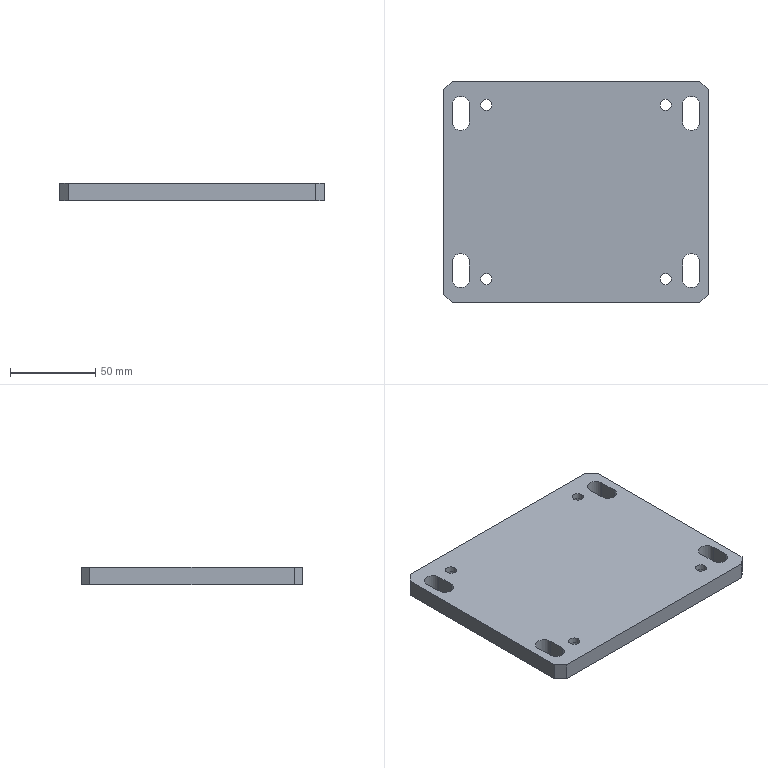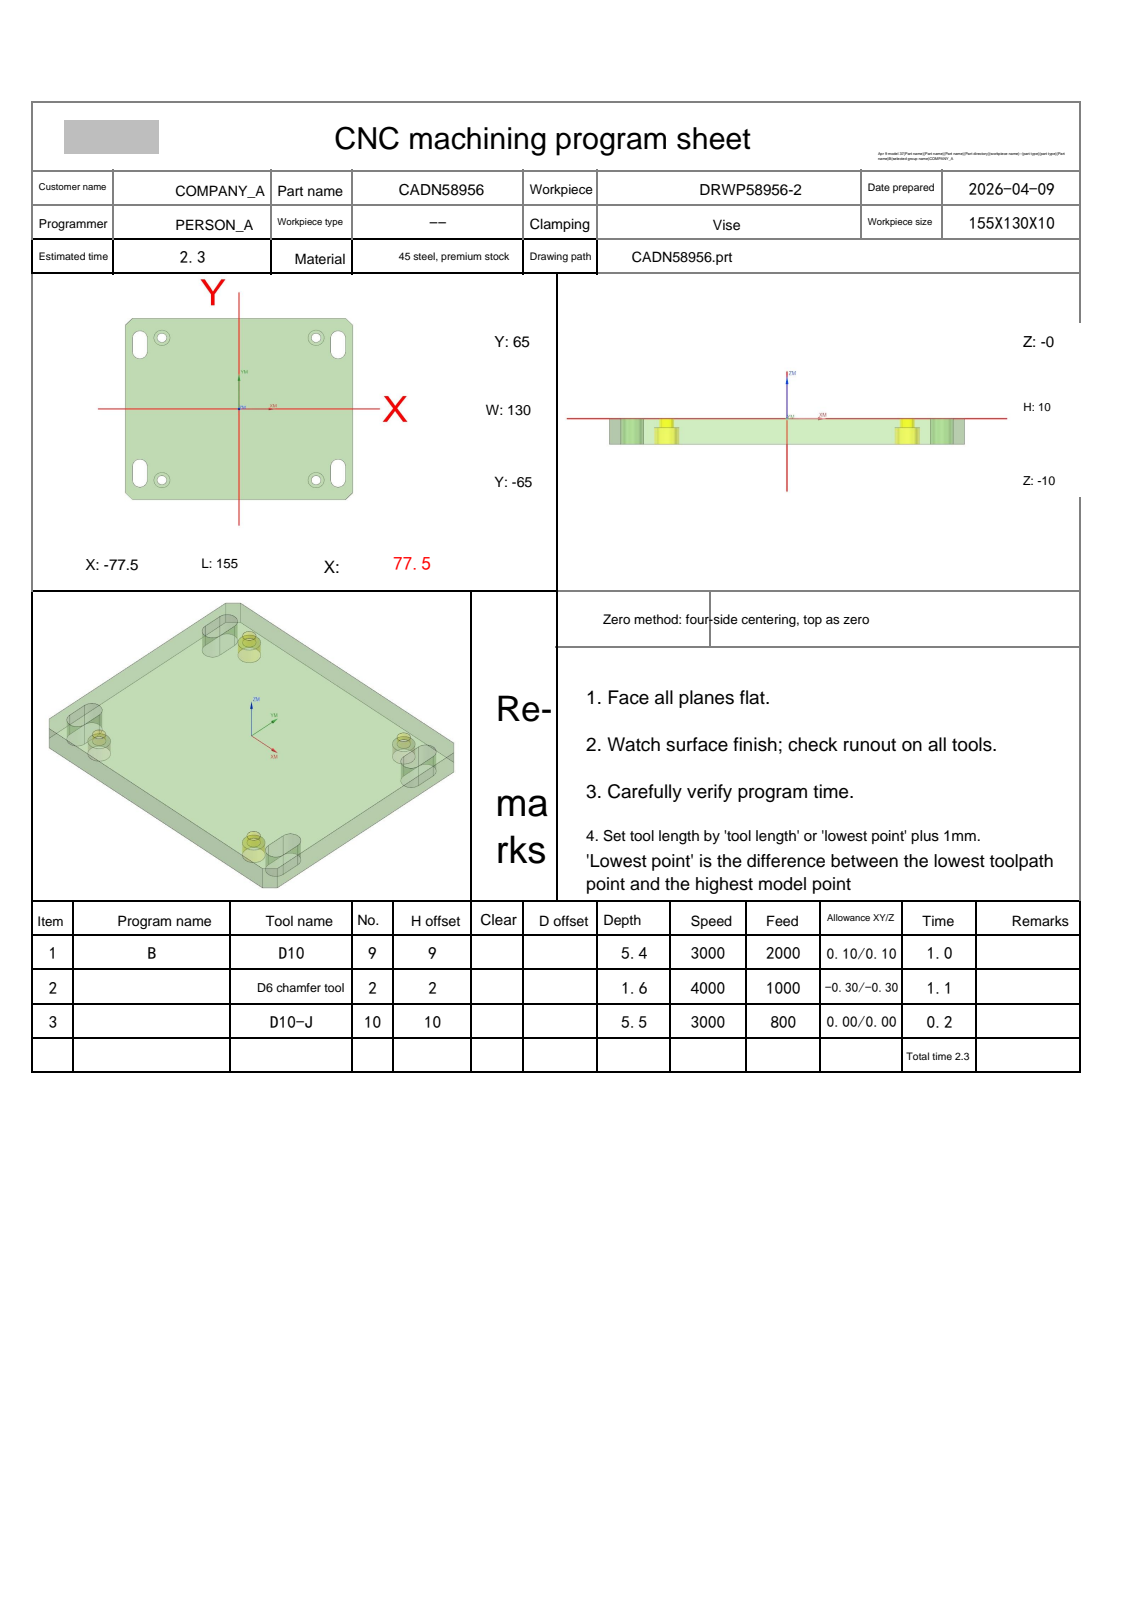NC program | NX | posted by the shop | part box 155 x 130 x 10 mm
Whole program:
%
O0001
(Machine time: 2.75 MIN)
(===Total Tool:3===)
(T9=D10     D=10.  R=0.   D-  H09 Z=-5.4  )
(T2=D6 chamfer tool   D=6.   R=0.   D-  H02 Z=-1.6  )
(T10=D10-J  D=10.  R=0.   D-  H10 Z=-5.5  )
G80 G90 G17 G49 G40
G91 G28 Z0
M01
N1 T09 M06
(D10  D=10. R=0. H=09 ce=0.10 di=0.10)
G00 G90 G54 X69.742 Y74.97 M03 S3000
G43 H09 Z20.
M08
Z-.3
G01 X76.106 Y68.606 F2000.
X81.106 Y63.606
X87.47 Y57.242
G00 Z-.6
G01 X81.106 Y63.606
X76.106 Y68.606
X69.742 Y74.97
G00 Z-.9
G01 X76.106 Y68.606
X81.106 Y63.606
X87.47 Y57.242
G00 Z-1.2
G01 X81.106 Y63.606
X76.106 Y68.606
X69.742 Y74.97
G00 Z-1.5
G01 X76.106 Y68.606
X81.106 Y63.606
X87.47 Y57.242
G00 Z-1.8
G01 X81.106 Y63.606
X76.106 Y68.606
X69.742 Y74.97
G00 Z-2.1
G01 X76.106 Y68.606
X81.106 Y63.606
X87.47 Y57.242
G00 Z-2.4
G01 X81.106 Y63.606
X76.106 Y68.606
X69.742 Y74.97
G00 Z-2.7
G01 X76.106 Y68.606
X81.106 Y63.606
X87.47 Y57.242
G00 Z-3.
G01 X81.106 Y63.606
X76.106 Y68.606
X69.742 Y74.97
G00 Z-3.3
G01 X76.106 Y68.606
X81.106 Y63.606
X87.47 Y57.242
G00 Z-3.6
G01 X81.106 Y63.606
X76.106 Y68.606
X69.742 Y74.97
G00 Z-3.9
G01 X76.106 Y68.606
X81.106 Y63.606
X87.47 Y57.242
G00 Z-4.2
G01 X81.106 Y63.606
X76.106 Y68.606
X69.742 Y74.97
G00 Z-4.5
G01 X76.106 Y68.606
X81.106 Y63.606
X87.47 Y57.242
G00 Z-4.8
G01 X81.106 Y63.606
X76.106 Y68.606
X69.742 Y74.97
G00 Z-5.1
G01 X76.106 Y68.606
X81.106 Y63.606
X87.47 Y57.242
G00 Z-5.4
G01 X81.106 Y63.606
X76.106 Y68.606
X69.742 Y74.97
G00 Z20.
X87.47 Y-57.242
Z-.3
G01 X81.106 Y-63.606
X76.106 Y-68.606
X69.742 Y-74.97
G00 Z-.6
G01 X76.106 Y-68.606
X81.106 Y-63.606
X87.47 Y-57.242
G00 Z-.9
G01 X81.106 Y-63.606
X76.106 Y-68.606
X69.742 Y-74.97
G00 Z-1.2
G01 X76.106 Y-68.606
X81.106 Y-63.606
X87.47 Y-57.242
G00 Z-1.5
G01 X81.106 Y-63.606
X76.106 Y-68.606
X69.742 Y-74.97
G00 Z-1.8
G01 X76.106 Y-68.606
X81.106 Y-63.606
X87.47 Y-57.242
G00 Z-2.1
G01 X81.106 Y-63.606
X76.106 Y-68.606
X69.742 Y-74.97
G00 Z-2.4
G01 X76.106 Y-68.606
X81.106 Y-63.606
X87.47 Y-57.242
G00 Z-2.7
G01 X81.106 Y-63.606
X76.106 Y-68.606
X69.742 Y-74.97
G00 Z-3.
G01 X76.106 Y-68.606
X81.106 Y-63.606
X87.47 Y-57.242
G00 Z-3.3
G01 X81.106 Y-63.606
X76.106 Y-68.606
X69.742 Y-74.97
G00 Z-3.6
G01 X76.106 Y-68.606
X81.106 Y-63.606
X87.47 Y-57.242
G00 Z-3.9
G01 X81.106 Y-63.606
X76.106 Y-68.606
X69.742 Y-74.97
G00 Z-4.2
G01 X76.106 Y-68.606
X81.106 Y-63.606
X87.47 Y-57.242
G00 Z-4.5
G01 X81.106 Y-63.606
X76.106 Y-68.606
X69.742 Y-74.97
G00 Z-4.8
G01 X76.106 Y-68.606
X81.106 Y-63.606
X87.47 Y-57.242
G00 Z-5.1
G01 X81.106 Y-63.606
X76.106 Y-68.606
X69.742 Y-74.97
G00 Z-5.4
G01 X76.106 Y-68.606
X81.106 Y-63.606
X87.47 Y-57.242
G00 Z20.
X-69.742 Y-74.97
Z-.3
G01 X-76.106 Y-68.606
X-81.106 Y-63.606
X-87.47 Y-57.242
G00 Z-.6
G01 X-81.106 Y-63.606
X-76.106 Y-68.606
X-69.742 Y-74.97
G00 Z-.9
G01 X-76.106 Y-68.606
X-81.106 Y-63.606
X-87.47 Y-57.242
G00 Z-1.2
G01 X-81.106 Y-63.606
X-76.106 Y-68.606
X-69.742 Y-74.97
G00 Z-1.5
G01 X-76.106 Y-68.606
X-81.106 Y-63.606
X-87.47 Y-57.242
G00 Z-1.8
G01 X-81.106 Y-63.606
X-76.106 Y-68.606
X-69.742 Y-74.97
G00 Z-2.1
G01 X-76.106 Y-68.606
X-81.106 Y-63.606
X-87.47 Y-57.242
G00 Z-2.4
G01 X-81.106 Y-63.606
X-76.106 Y-68.606
X-69.742 Y-74.97
G00 Z-2.7
G01 X-76.106 Y-68.606
X-81.106 Y-63.606
X-87.47 Y-57.242
G00 Z-3.
G01 X-81.106 Y-63.606
X-76.106 Y-68.606
X-69.742 Y-74.97
G00 Z-3.3
G01 X-76.106 Y-68.606
X-81.106 Y-63.606
X-87.47 Y-57.242
G00 Z-3.6
G01 X-81.106 Y-63.606
X-76.106 Y-68.606
X-69.742 Y-74.97
G00 Z-3.9
G01 X-76.106 Y-68.606
X-81.106 Y-63.606
X-87.47 Y-57.242
G00 Z-4.2
G01 X-81.106 Y-63.606
X-76.106 Y-68.606
X-69.742 Y-74.97
G00 Z-4.5
G01 X-76.106 Y-68.606
X-81.106 Y-63.606
X-87.47 Y-57.242
G00 Z-4.8
G01 X-81.106 Y-63.606
X-76.106 Y-68.606
X-69.742 Y-74.97
G00 Z-5.1
G01 X-76.106 Y-68.606
X-81.106 Y-63.606
X-87.47 Y-57.242
G00 Z-5.4
G01 X-81.106 Y-63.606
X-76.106 Y-68.606
X-69.742 Y-74.97
G00 Z20.
X-87.47 Y57.242
Z-.3
G01 X-81.106 Y63.606
X-76.106 Y68.606
X-69.742 Y74.97
G00 Z-.6
G01 X-76.106 Y68.606
X-81.106 Y63.606
X-87.47 Y57.242
G00 Z-.9
G01 X-81.106 Y63.606
X-76.106 Y68.606
X-69.742 Y74.97
G00 Z-1.2
G01 X-76.106 Y68.606
X-81.106 Y63.606
X-87.47 Y57.242
G00 Z-1.5
G01 X-81.106 Y63.606
X-76.106 Y68.606
X-69.742 Y74.97
G00 Z-1.8
G01 X-76.106 Y68.606
X-81.106 Y63.606
X-87.47 Y57.242
G00 Z-2.1
G01 X-81.106 Y63.606
X-76.106 Y68.606
X-69.742 Y74.97
G00 Z-2.4
G01 X-76.106 Y68.606
X-81.106 Y63.606
X-87.47 Y57.242
G00 Z-2.7
G01 X-81.106 Y63.606
X-76.106 Y68.606
X-69.742 Y74.97
G00 Z-3.
G01 X-76.106 Y68.606
X-81.106 Y63.606
X-87.47 Y57.242
G00 Z-3.3
G01 X-81.106 Y63.606
X-76.106 Y68.606
X-69.742 Y74.97
G00 Z-3.6
G01 X-76.106 Y68.606
X-81.106 Y63.606
X-87.47 Y57.242
G00 Z-3.9
G01 X-81.106 Y63.606
X-76.106 Y68.606
X-69.742 Y74.97
G00 Z-4.2
G01 X-76.106 Y68.606
X-81.106 Y63.606
X-87.47 Y57.242
G00 Z-4.5
G01 X-81.106 Y63.606
X-76.106 Y68.606
X-69.742 Y74.97
G00 Z-4.8
G01 X-76.106 Y68.606
X-81.106 Y63.606
X-87.47 Y57.242
G00 Z-5.1
G01 X-81.106 Y63.606
X-76.106 Y68.606
X-69.742 Y74.97
G00 Z-5.4
G01 X-76.106 Y68.606
X-81.106 Y63.606
X-87.47 Y57.242
G00 Z20.
G91 G28 Z0.0
M05
M09
G91 G28 Z0.0
M01
N2 T02 M06
(D6 chamfer tool  D=6. R=0. H=02 ce=-0.30 di=-0.80)
G00 G90 G54 X-52.227 Y50.09 M03 S4000
G43 H02 Z20.
M08
Z-1.1
G01 Z-1.6 F600.
X-52.05 Y49.5
G03 X-50.55 Y51. I0.0 J1.5
X-52.5 Y52.95 I-1.95 J0.0
X-54.45 Y51. I0.0 J-1.95
X-52.5 Y49.05 I1.95 J0.0
X-50.55 Y51. I0.0 J1.95
X-52.05 Y52.5 I-1.5 J0.0
G01 X-52.227 Y51.91
Z-1.1
G00 Z20.
Y-51.91
Z-1.1
G01 Z-1.6
X-52.05 Y-52.5
G03 X-50.55 Y-51. I0.0 J1.5
X-52.5 Y-49.05 I-1.95 J0.0
X-54.45 Y-51. I0.0 J-1.95
X-52.5 Y-52.95 I1.95 J0.0
X-50.55 Y-51. I0.0 J1.95
X-52.05 Y-49.5 I-1.5 J0.0
G01 X-52.227 Y-50.09
Z-1.1
G00 Z20.
X52.773 Y-51.91
Z-1.1
G01 Z-1.6
X52.95 Y-52.5
G03 X54.45 Y-51. I0.0 J1.5
X52.5 Y-49.05 I-1.95 J0.0
X50.55 Y-51. I0.0 J-1.95
X52.5 Y-52.95 I1.95 J0.0
X54.45 Y-51. I0.0 J1.95
X52.95 Y-49.5 I-1.5 J0.0
G01 X52.773 Y-50.09
Z-1.1
G00 Z20.
Y50.09
Z-1.1
G01 Z-1.6
X52.95 Y49.5
G03 X54.45 Y51. I0.0 J1.5
X52.5 Y52.95 I-1.95 J0.0
X50.55 Y51. I0.0 J-1.95
X52.5 Y49.05 I1.95 J0.0
X54.45 Y51. I0.0 J1.95
X52.95 Y52.5 I-1.5 J0.0
G01 X52.773 Y51.91
Z-1.1
G00 Z20.
G00 G90 X.386 Y-66.227 M03 S3500
Z20.
Z.172
G01 Z-1.199 F1000.
G03 X.1 Y-66.027 I-1.286 J-1.532
G01 X.054 Y-65.997
X0.0 Y-66.
X-72.5
X-72.759 Y-65.966
X-73. Y-65.866
X-73.207 Y-65.707
X-78.207 Y-60.707
X-78.366 Y-60.5
X-78.466 Y-60.259
X-78.5 Y-60.
Y60.
X-78.466 Y60.259
X-78.366 Y60.5
X-78.207 Y60.707
X-73.207 Y65.707
X-73. Y65.866
X-72.759 Y65.966
X-72.5 Y66.
X72.5
X72.759 Y65.966
X73. Y65.866
X73.207 Y65.707
X78.207 Y60.707
X78.366 Y60.5
X78.466 Y60.259
X78.5 Y60.
Y-60.
X78.466 Y-60.259
X78.366 Y-60.5
X78.207 Y-60.707
X73.207 Y-65.707
X73. Y-65.866
X72.759 Y-65.966
X72.5 Y-66.
X0.0
X-.054 Y-65.997
X-.1 Y-66.027
G03 X-.386 Y-66.227 I1. J-1.732
G01 Z.172
G00 Z10.
X-50.442 Y-51.404
Z.249
G01 Z-1.199
G03 X-50.268 Y-51.102 I-1.638 J1.147
G01 X-50.242 Y-51.054
X-50.25 Y-51.
G03 X-52.5 Y-48.75 I-2.25 J0.0
X-54.75 Y-51. I0.0 J-2.25
X-52.5 Y-53.25 I2.25 J0.0
X-50.25 Y-51. I0.0 J2.25
G01 X-50.242 Y-50.946
X-50.268 Y-50.898
G03 X-50.442 Y-50.596 I-1.813 J-.845
G01 Z.255
G00 Z10.
X-63.727 Y-46.386
Z.172
G01 Z-1.199
G03 X-63.527 Y-46.1 I-1.532 J1.286
G01 X-63.497 Y-46.054
X-63.5 Y-46.
Y-41.
G03 X-67.5 Y-37. I-4. J0.0
X-71.5 Y-41. I0.0 J-4.
G01 Y-51.
G03 X-67.5 Y-55. I4. J0.0
X-63.5 Y-51. I0.0 J4.
G01 Y-46.
X-63.497 Y-45.946
X-63.527 Y-45.9
G03 X-63.727 Y-45.614 I-1.732 J-1.
G01 Z.172
G00 Z10.
Y45.614
Z.172
G01 Z-1.199
G03 X-63.527 Y45.9 I-1.532 J1.286
G01 X-63.497 Y45.946
X-63.5 Y46.
Y51.
G03 X-67.5 Y55. I-4. J0.0
X-71.5 Y51. I0.0 J-4.
G01 Y41.
G03 X-67.5 Y37. I4. J0.0
X-63.5 Y41. I0.0 J4.
G01 Y46.
X-63.497 Y46.054
X-63.527 Y46.1
G03 X-63.727 Y46.386 I-1.732 J-1.
G01 Z.172
G00 Z10.
X-50.442 Y50.596
Z.249
G01 Z-1.199
G03 X-50.268 Y50.898 I-1.638 J1.147
G01 X-50.242 Y50.946
X-50.25 Y51.
G03 X-52.5 Y53.25 I-2.25 J0.0
X-54.75 Y51. I0.0 J-2.25
X-52.5 Y48.75 I2.25 J0.0
X-50.25 Y51. I0.0 J2.25
G01 X-50.242 Y51.054
X-50.268 Y51.102
G03 X-50.442 Y51.404 I-1.813 J-.845
G01 Z.255
G00 Z10.
X54.558 Y50.596
Z.255
G01 Z-1.199
G03 X54.732 Y50.898 I-1.638 J1.147
G01 X54.758 Y50.946
X54.75 Y51.
G03 X52.5 Y53.25 I-2.25 J0.0
X50.25 Y51. I0.0 J-2.25
X52.5 Y48.75 I2.25 J0.0
X54.75 Y51. I0.0 J2.25
G01 X54.758 Y51.054
X54.732 Y51.102
G03 X54.558 Y51.404 I-1.813 J-.845
G01 Z.249
G00 Z2.551
X63.727 Y46.386
Z.172
G01 Z-1.199
G03 X63.527 Y46.1 I1.532 J-1.286
G01 X63.497 Y46.054
X63.5 Y46.
Y41.
G03 X67.5 Y37. I4. J0.0
X71.5 Y41. I0.0 J4.
G01 Y51.
G03 X67.5 Y55. I-4. J0.0
X63.5 Y51. I0.0 J-4.
G01 Y46.
X63.497 Y45.946
X63.527 Y45.9
G03 X63.727 Y45.614 I1.732 J1.
G01 Z.172
G00 Z10.
X71.273 Y-46.386
Z.172
G01 Z-1.199
G03 X71.473 Y-46.1 I-1.532 J1.286
G01 X71.503 Y-46.054
X71.5 Y-46.
Y-41.
G03 X67.5 Y-37. I-4. J0.0
X63.5 Y-41. I0.0 J-4.
G01 Y-51.
G03 X67.5 Y-55. I4. J0.0
X71.5 Y-51. I0.0 J4.
G01 Y-46.
X71.503 Y-45.946
X71.473 Y-45.9
G03 X71.273 Y-45.614 I-1.732 J-1.
G01 Z.172
G00 Z10.
X54.558 Y-51.404
Z.255
G01 Z-1.199
G03 X54.732 Y-51.102 I-1.638 J1.147
G01 X54.758 Y-51.054
X54.75 Y-51.
G03 X52.5 Y-48.75 I-2.25 J0.0
X50.25 Y-51. I0.0 J-2.25
X52.5 Y-53.25 I2.25 J0.0
X54.75 Y-51. I0.0 J2.25
G01 X54.758 Y-50.946
X54.732 Y-50.898
G03 X54.558 Y-50.596 I-1.813 J-.845
G01 Z.249
G00 Z20.
G91 G28 Z0.0
M05
M09
G91 G28 Z0.0
M01
N3 T10 M06
(D10-J  D=10. R=0. H=10 ce=0.00 di=0.00)
G00 G90 G54 X-71.793 Y-72.778 M03 S3000
G43 H10 Z20.
M08
Z-4.5
G01 Z-5.5 F800.
X-76.036 Y-68.536
X-81.036 Y-63.536
X-85.278 Y-59.293
Z-4.5
G00 Z20.
Y59.293
Z-4.5
G01 Z-5.5
X-81.036 Y63.536
X-76.036 Y68.536
X-71.793 Y72.778
Z-4.5
G00 Z20.
X71.793
Z-4.5
G01 Z-5.5
X76.036 Y68.536
X81.036 Y63.536
X85.278 Y59.293
Z-4.5
G00 Z20.
Y-59.293
Z-4.5
G01 Z-5.5
X81.036 Y-63.536
X76.036 Y-68.536
X71.793 Y-72.778
Z-4.5
G00 Z20.
M05
M09
G91 G28 Z0.0
G91 G28 Y0.0
M30
%